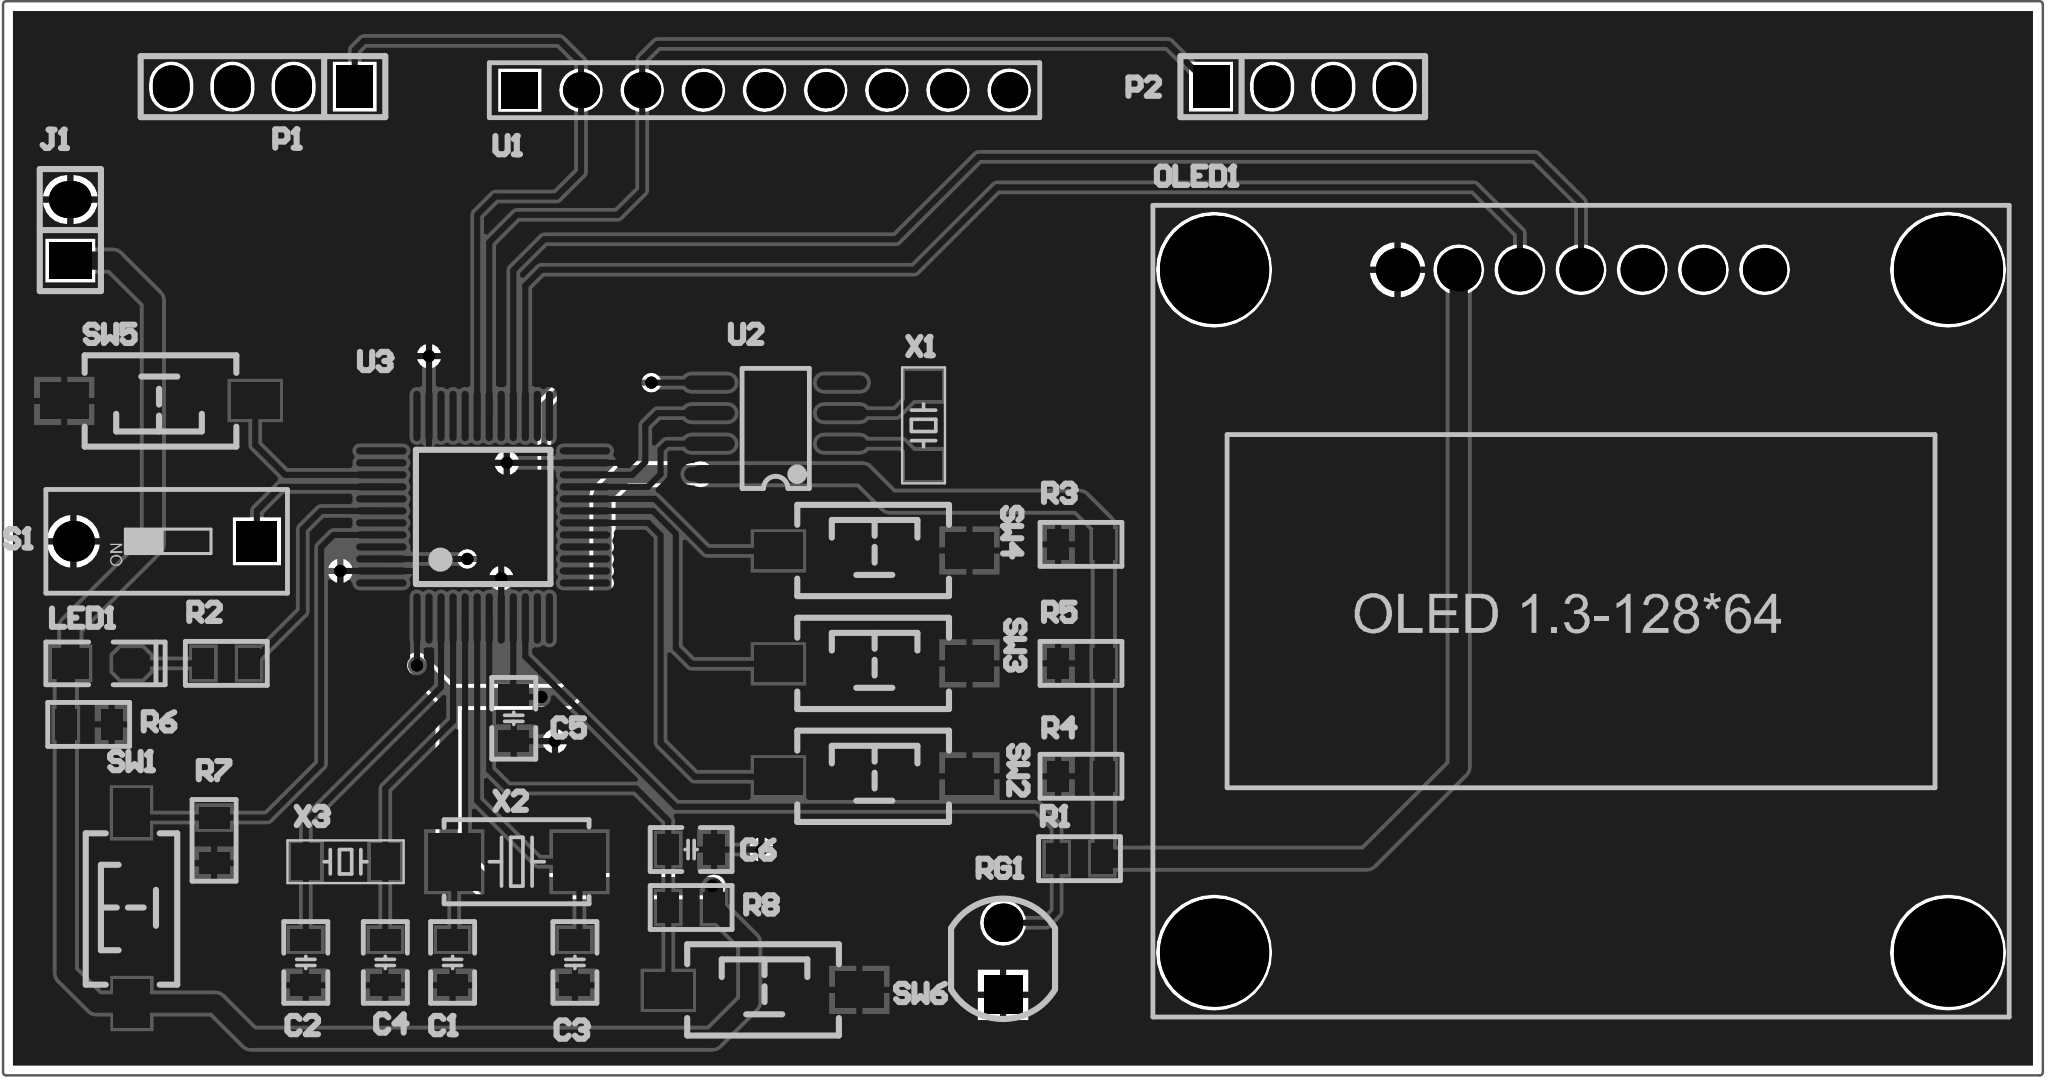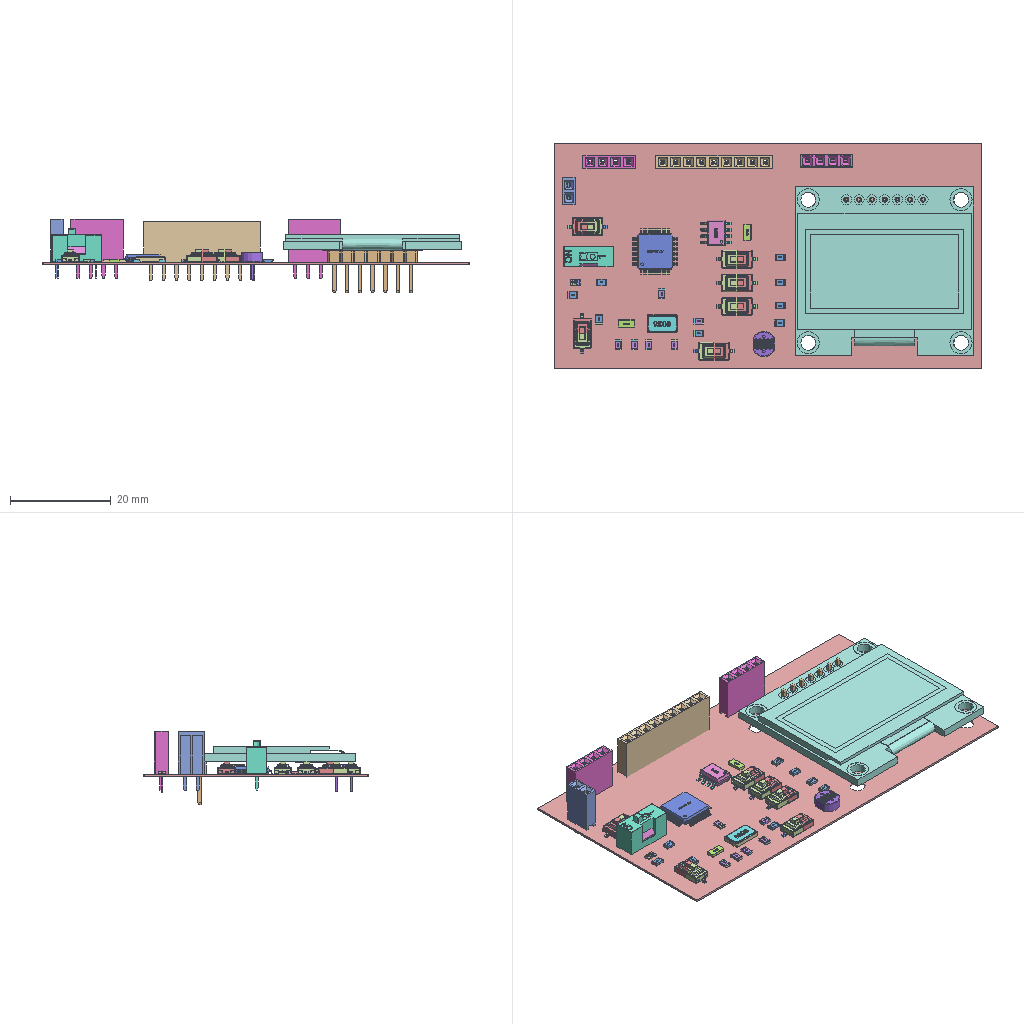Circuit board layout | Altium Designer | box 84.7 x 44.7 x 14.5 mm
Layer stack:
# Altium Designer layer stack of  (unit mm; dielectric type: 0 none, 1 core, 2 prepreg, 3 surface material)
index,name,kind,layer,copper_thickness_mm,dielectric_type,dielectric_thickness_mm,dielectric_material,dielectric_constant
0,Top Paste,other,,,,,,
1,Top Overlay,other,,,,,,
2,Top Solder,dielectric,,,3,0.0102,Solder Resist,3.5
3,Top Layer,copper,Top Layer,0.0356,,,,
4,Dielectric 1,dielectric,,,0,0.32,FR-4,4.8
5,Bottom Layer,copper,Bottom Layer,0.0356,,,,
6,Bottom Solder,dielectric,,,3,0.0102,Solder Resist,3.5
7,Bottom Overlay,other,,,,,,
8,Bottom Paste,other,,,,,,
# drill layer pairs: low layer,high layer
drill_pair,Top Layer,Bottom Layer
Part placement:
Designator,Comment,Layer,Footprint,Center-X(mm),Center-Y(mm),Rotation
J1,Female HDR1X2,TopLayer,Fe-HDR1X2/2.54-S,74.422,83.312,90
X3,32.768K,TopLayer,OSC_3215-2P,85.852,57.023,180
X2,8MHz,TopLayer,OSC_6035-2P,92.964,57.023,180
X1,32.768K,TopLayer,OSC_3215-2P,109.855,75.184,270
U3,STM32F103C8T6,TopLayer,LQFP48_7X7,91.567,71.361,360
U2,DS1302,TopLayer,SOP8,103.715,75.057,180
U1,COMPIM,TopLayer,Fe-HDR1X9/2.54-S,103.251,89.134,90
SW6,3x6x5,TopLayer,TSW_SMD-3*6*2.5,103.222,51.679,360
SW5,3x6x5,TopLayer,TSW_SMD-3*6*2.5,78.134,76.21,180
SW4,3x6x5,TopLayer,TSW_SMD-3*6*2.5,107.794,69.967,360
SW3,3x6x5,TopLayer,TSW_SMD-3*6*2.5,107.794,65.268,360
SW2,3x6x5,TopLayer,TSW_SMD-3*6*2.5,107.794,60.569,360
SW1,3x6x5,TopLayer,TSW_SMD-3*6*2.5,76.972,55.089,90
S1,KCD1-101,TopLayer,CSW_DIP-1P,78.359,70.358,90
RG1,10K,TopLayer,RG5528,113.157,52.983,90
R8,10K,TopLayer,R_0805_L,100.203,55.118,0
R7,10K,TopLayer,R_0805_L,80.391,57.912,90
R6,10K,TopLayer,R_0805_L,75.184,62.738,180
R5,10K,TopLayer,R_0805_L,116.393,65.278,0
R4,10K,TopLayer,R_0805_L,116.393,60.579,0
R3,10K,TopLayer,R_0805_L,116.393,70.231,0
R2,10R,TopLayer,R_0805_L,80.899,65.278,0
R1,10K,TopLayer,R_0805_L,116.332,57.15,360
P2,Header 4,TopLayer,Fe-HDR1X4/2.54-S,125.603,89.281,90
P1,Header 4,TopLayer,Fe-HDR1X4/2.54-S,82.423,89.281,270
OLED1,OLED 1.3-12864_7pin,TopLayer,OLED_1.3-12864_7pin,137.16,67.451,0
LED1,Red,TopLayer,LED_0805G,75.692,65.278,360
C6,100nF,TopLayer,C_0805_L,100.203,57.531,0
C5,100nF,TopLayer,C_0805_L,92.837,62.992,270
C4,22pF,TopLayer,C_0805_L,87.503,52.832,270
C3,22pF,TopLayer,C_0805_L,95.377,52.832,90
C2,22pF,TopLayer,C_0805_L,84.201,52.832,270
C1,22pF,TopLayer,C_0805_L,90.297,52.832,90
Pad and via stacks:
# Altium Designer via and pad stacks of  (unit mm). Each distinct definition once, with the count of objects using it.
# via: kind,start_layer,end_layer,hole_mm,diameter_mm,mode(0 simple;1 top-mid-bottom;2 full stack),diameter_per_layer,count,example_net
# pad: kind,layer,hole_mm,hole_type(0 round;1 square;2 slot),plating,top_size,top_shape(1 round;2 rect;3 octagon;9 rounded rect),mid_size,bottom_size,mode,footprint,size_per_layer,count,example
pad,Top Layer,0,0,plated,1.27x0.889,2,1.27x0.889,1.27x0.889,0,C 0805_L,,12,C6.1
pad,Top Layer,0,0,plated,2x1.5,2,2x1.5,2x1.5,0,TSW SMD-3*6*2.5,,12,SW6.1
pad,Top Layer,0,0,plated,1.27x0.889,2,1.27x0.889,1.27x0.889,0,R 0805_L,,16,R8.1
pad,Top Layer,0,0,plated,1.2x1.5,2,1.2x1.5,1.2x1.5,0,OSC 3215-2P,,4,X3.1
pad,Top Layer,0,0,unplated,2.4x2.2,2,2.4x2.2,2.4x2.2,0,OSC 6035-2P,,2,X2.1
pad,Top Layer,0,0,plated,1.524x1.27,2,1.524x1.27,1.524x1.27,0,LED 0805G,,1,LED1.1
pad,Top Layer,0,0,plated,1.524x1.27,3,1.524x1.27,1.524x1.27,0,LED 0805G,,1,LED1.2
pad,Top Layer,0,0,plated,0.3x2.1,1,0.3x2.1,0.3x2.1,0,LQFP48 7X7,,48,U3.48
pad,Top Layer,0,0,plated,0.6x2.1,1,0.6x2.1,0.6x2.1,0,SOP8,,7,U2.5
pad,Top Layer,0,0,plated,0.6x2.1,2,0.6x2.1,0.6x2.1,0,SOP8,,1,U2.1
pad,Multi-Layer,0.9,0,plated,1.7x1.7,2,1.7x1.7,1.7x1.7,0,CSW DIP-1P,,1,S1.1
pad,Multi-Layer,0.9,0,plated,1.7x1.7,1,1.7x1.7,1.7x1.7,0,CSW DIP-1P,,1,S1.2
pad,Multi-Layer,0.8,0,plated,1.6x1.6,2,1.6x1.6,1.6x1.6,0,RG5528,,1,RG1.1
pad,Multi-Layer,0.8,0,plated,1.6x1.6,1,1.6x1.6,1.6x1.6,0,RG5528,,1,RG1.2
pad,Multi-Layer,0.8,0,plated,1.8x1.8,1,1.8x1.8,1.8x1.8,0,OLED 1.3-12864_7pin,,7,OLED1.1
pad,Multi-Layer,3,0,plated,4.5x4.5,1,4.5x4.5,4.5x4.5,0,OLED 1.3-12864_7pin,,4,OLED1.0
pad,Multi-Layer,0.8128,0,plated,1.524x1.778,2,1.524x1.778,1.524x1.778,0,Fe-HDR1X2/2.54-S,,1,J1.1
pad,Multi-Layer,0.8128,0,plated,1.524x1.778,1,1.524x1.778,1.524x1.778,0,Fe-HDR1X2/2.54-S,,1,J1.2
pad,Multi-Layer,0.9,0,plated,1.5x1.5,2,1.5x1.5,1.5x1.5,0,Fe-HDR1X9/2.54-S,,1,U1.1
pad,Multi-Layer,0.9,0,plated,1.5x1.5,1,1.5x1.5,1.5x1.5,0,Fe-HDR1X9/2.54-S,,8,U1.3
pad,Multi-Layer,0.8128,0,plated,1.524x1.778,1,1.524x1.778,1.524x1.778,0,Fe-HDR1X4/2.54-S,,6,P2.4
pad,Multi-Layer,0.8128,0,plated,1.524x1.778,2,1.524x1.778,1.524x1.778,0,Fe-HDR1X4/2.54-S,,2,P2.1
via,Top Layer,Bottom Layer,0.254,0.508,0,,12,GND
Copper pours:
name,layer,net,type(0 solid;1 hatched;2 none)
D,Top Layer,GND,0
D,Bottom Layer,GND,0
Design rules, without the lines most boards share:
# Altium Designer design rules of  (exported by Altium Designer, unit mm)
# columns: name | kind | enabled | priority | scope1 | scope2 | descriptor | typed fields (field=value)
SilkToSilkClearance | 55 | enabled | 1 | All | All | Silk to Silk (Clearance=0mil) (All),(All) |
SilkToSolderMaskClearance | 54 | enabled | 1 | IsPad | All | Silk To Solder Mask (Clearance=0mil) (IsPad),(All) |
MinimumSolderMaskSliver | 53 | enabled | 1 | All | All | Minimum Solder Mask Sliver (Gap=0mil) (All),(All) |
HoleToHoleClearance | 52 | enabled | 1 | All | All | Hole To Hole Clearance (Gap=10mil) (All),(All) | gap=0.254
DiffPairsRouting | 51 | enabled | 1 | All | All | Differential Pairs Uncoupled Length using the Gap Constraints (Min=10mil) (Max=10mil) (Prefered=10mil)  and Width Constraints (Min=15mil) (Max=15mil) (Prefered=15mil) (All) |
HoleSize | 42 | enabled | 1 | All | All | Hole Size Constraint (Min=1mil) (Max=77777mil) (All) |
SolderMaskExpansion | 13 | enabled | 1 | All | All | Solder Mask Expansion (Expansion =4mil) (All) | expansion=0.1016
PasteMaskExpansion | 14 | enabled | 1 | All | All | Paste Mask Expansion (Expansion =0mil) (All) | expansion=0
RoutingVias | 11 | enabled | 1 | All | All | Routing Via (MinHoleWidth=28mil) (MaxHoleWidth=28mil) (PreferredHoleWidth=28mil) (MinWidth=50mil) (MaxWidth=50mil) (PreferedWidth=50mil) (All) | via_min_hole=0.7112 via_max_hole=0.7112 via_preferred_diameter=1.27 via_preferred_hole=0.7112
Width | 2 | enabled | 1 | All | All | Width Constraint (Min=10mil) (Max=30mil) (Preferred=10mil) (All) |
PolygonConnect | 20 | enabled | 1 | All | All | Polygon Connect Rule(Relief Connect )(Conductor Width=10mil) (Relief Angle=90 Angle) (Entries=4) (Air Gap Width=10mil) (All),(All) | connect_style(0=relief,1=direct,2=none)=0 relief_conductor_width=0.254 relief_entries=4
PlaneConnect | 6 | enabled | 1 | All | All | Power Plane Connect Rule(Relief Connect )(Expansion=20mil) (Conductor Width=10mil) (Air Gap=10mil) (Entries=4) (All) | relief_conductor_width=0.254 relief_entries=4 relief_expansion=0.508
Clearance | 0 | enabled | 1 | All | All | Clearance Constraint (Gap=6mil) (All),(All) | gap=0.1524
Classes set for this board:
# Altium Designer classes of  (member kind: 0 net, 1 component, 2 from-to, 3 pad, 4 layer, 5 differential pair, 6 design channel, 7 polygon, 8 structure, 9 xSignal)
# columns: class name | member kind | superclass | members
Sheet1 | 1 | no | C1; C2; C3; C4; C5; C6; LED1; OLED1; P1; P2; R1; R2; R3; R4; R5; R6; R7; R8; RG1; S1; SW1; SW2; SW3; SW4; SW5; SW6; U1; U2; U3; X1; X2; X3; J1;